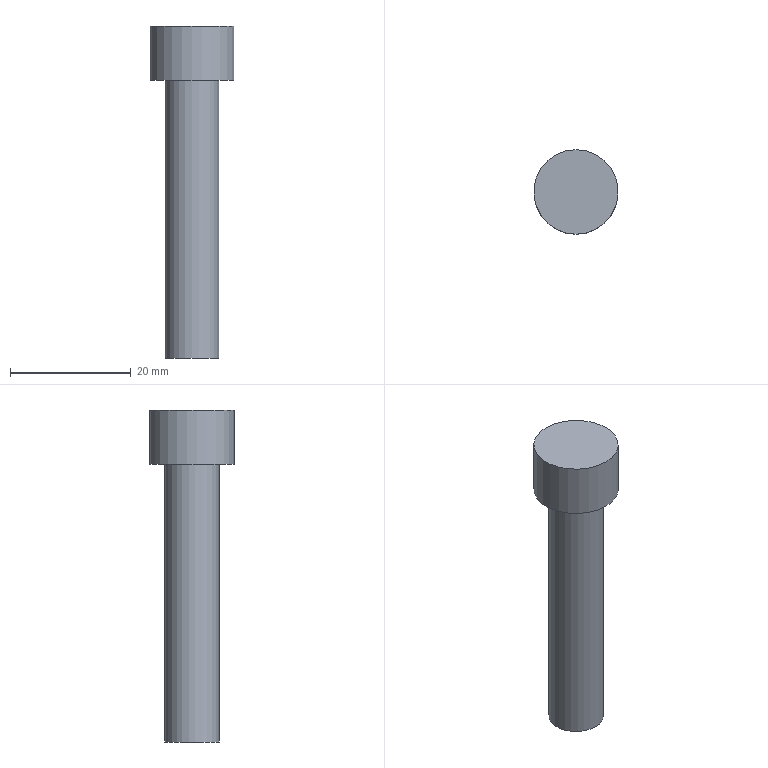Part | STEP file | SOLID | 1 solid | 5 faces | box 14 x 14 x 55 mm | volume 4312 mm3 | plane 3 | cylinder 2 | commonest cylinder face diameters 9 x1 14 x1
STEP:
#1=CARTESIAN_POINT('',(0.,0.,0.));
#2=DIRECTION('',(0.,0.,1.));
#3=DIRECTION('',(1.,0.,0.));
#4=AXIS2_PLACEMENT_3D('',#1,#2,#3);
#5=CARTESIAN_POINT('',(0.,-4.5,-55.));
#6=VERTEX_POINT('',#5);
#7=CARTESIAN_POINT('',(0.,0.,-55.));
#8=DIRECTION('',(0.,0.,1.));
#9=DIRECTION('',(0.,-1.,0.));
#10=AXIS2_PLACEMENT_3D('',#7,#8,#9);
#11=CIRCLE('',#10,4.5);
#12=CARTESIAN_POINT('',(0.,0.,-55.));
#13=DIRECTION('',(0.,0.,1.));
#14=DIRECTION('',(0.,-1.,0.));
#15=AXIS2_PLACEMENT_3D('',#12,#13,#14);
#16=PLANE('',#15);
#17=CARTESIAN_POINT('',(0.,0.));
#18=DIRECTION('',(1.,0.));
#19=AXIS2_PLACEMENT_2D('',#17,#18);
#20=CIRCLE('',#19,4.5);
#21=(GEOMETRIC_REPRESENTATION_CONTEXT(2)PARAMETRIC_REPRESENTATION_CONTEXT()REPRESENTATION_CONTEXT('',''));
#22=DEFINITIONAL_REPRESENTATION('',(#20),#21);
#23=PCURVE('',#16,#22);
#24=CARTESIAN_POINT('',(0.,0.,1.));
#25=DIRECTION('',(0.,0.,1.));
#26=DIRECTION('',(0.,-1.,0.));
#27=AXIS2_PLACEMENT_3D('',#24,#25,#26);
#28=CYLINDRICAL_SURFACE('',#27,4.5);
#29=CARTESIAN_POINT('',(0.,-56.));
#30=DIRECTION('',(1.,0.));
#31=VECTOR('',#30,1.);
#32=LINE('',#29,#31);
#33=(GEOMETRIC_REPRESENTATION_CONTEXT(2)PARAMETRIC_REPRESENTATION_CONTEXT()REPRESENTATION_CONTEXT('',''));
#34=DEFINITIONAL_REPRESENTATION('',(#32),#33);
#35=PCURVE('',#28,#34);
#36=SURFACE_CURVE('',#11,(#23,#35),.PCURVE_S1.);
#37=EDGE_CURVE('',#6,#6,#36,.T.);
#38=ORIENTED_EDGE('',*,*,#37,.F.);
#39=EDGE_LOOP('',(#38));
#40=FACE_BOUND('',#39,.T.);
#41=ADVANCED_FACE('',(#40),#16,.F.);
#42=ORIENTED_EDGE('',*,*,#37,.T.);
#43=CARTESIAN_POINT('',(0.,-4.5,-9.));
#44=VERTEX_POINT('',#43);
#45=CARTESIAN_POINT('',(0.,-4.5,-55.));
#46=CARTESIAN_POINT('',(0.,-4.5,-9.));
#47=B_SPLINE_CURVE_WITH_KNOTS('',1,(#45,#46),.UNSPECIFIED.,.F.,.F.,(2,2),(-56.,-10.),.PIECEWISE_BEZIER_KNOTS.);
#48=CARTESIAN_POINT('',(6.283,0.));
#49=DIRECTION('',(0.,1.));
#50=VECTOR('',#49,1.);
#51=LINE('',#48,#50);
#52=(GEOMETRIC_REPRESENTATION_CONTEXT(2)PARAMETRIC_REPRESENTATION_CONTEXT()REPRESENTATION_CONTEXT('',''));
#53=DEFINITIONAL_REPRESENTATION('',(#51),#52);
#54=PCURVE('',#28,#53);
#55=CARTESIAN_POINT('',(0.,0.));
#56=DIRECTION('',(0.,1.));
#57=VECTOR('',#56,1.);
#58=LINE('',#55,#57);
#59=(GEOMETRIC_REPRESENTATION_CONTEXT(2)PARAMETRIC_REPRESENTATION_CONTEXT()REPRESENTATION_CONTEXT('',''));
#60=DEFINITIONAL_REPRESENTATION('',(#58),#59);
#61=PCURVE('',#28,#60);
#62=SEAM_CURVE('',#47,(#54,#61),.PCURVE_S1.);
#63=EDGE_CURVE('',#6,#44,#62,.T.);
#64=ORIENTED_EDGE('',*,*,#63,.T.);
#65=CARTESIAN_POINT('',(0.,0.,-9.));
#66=DIRECTION('',(0.,0.,1.));
#67=DIRECTION('',(0.,-1.,0.));
#68=AXIS2_PLACEMENT_3D('',#65,#66,#67);
#69=CIRCLE('',#68,4.5);
#70=CARTESIAN_POINT('',(0.,-10.));
#71=DIRECTION('',(1.,0.));
#72=VECTOR('',#71,1.);
#73=LINE('',#70,#72);
#74=(GEOMETRIC_REPRESENTATION_CONTEXT(2)PARAMETRIC_REPRESENTATION_CONTEXT()REPRESENTATION_CONTEXT('',''));
#75=DEFINITIONAL_REPRESENTATION('',(#73),#74);
#76=PCURVE('',#28,#75);
#77=CARTESIAN_POINT('',(0.,0.,-9.));
#78=DIRECTION('',(0.,0.,1.));
#79=DIRECTION('',(0.,-1.,0.));
#80=AXIS2_PLACEMENT_3D('',#77,#78,#79);
#81=PLANE('',#80);
#82=CARTESIAN_POINT('',(0.,0.));
#83=DIRECTION('',(1.,0.));
#84=AXIS2_PLACEMENT_2D('',#82,#83);
#85=CIRCLE('',#84,4.5);
#86=(GEOMETRIC_REPRESENTATION_CONTEXT(2)PARAMETRIC_REPRESENTATION_CONTEXT()REPRESENTATION_CONTEXT('',''));
#87=DEFINITIONAL_REPRESENTATION('',(#85),#86);
#88=PCURVE('',#81,#87);
#89=SURFACE_CURVE('',#69,(#76,#88),.PCURVE_S1.);
#90=EDGE_CURVE('',#44,#44,#89,.T.);
#91=ORIENTED_EDGE('',*,*,#90,.F.);
#92=ORIENTED_EDGE('',*,*,#63,.F.);
#93=EDGE_LOOP('',(#42,#64,#91,#92));
#94=FACE_BOUND('',#93,.T.);
#95=ADVANCED_FACE('',(#94),#28,.T.);
#96=CARTESIAN_POINT('',(0.,-7.,-9.));
#97=VERTEX_POINT('',#96);
#98=CARTESIAN_POINT('',(0.,0.,-9.));
#99=DIRECTION('',(0.,0.,1.));
#100=DIRECTION('',(0.,-1.,0.));
#101=AXIS2_PLACEMENT_3D('',#98,#99,#100);
#102=CIRCLE('',#101,7.);
#103=CARTESIAN_POINT('',(0.,0.));
#104=DIRECTION('',(1.,0.));
#105=AXIS2_PLACEMENT_2D('',#103,#104);
#106=CIRCLE('',#105,7.);
#107=(GEOMETRIC_REPRESENTATION_CONTEXT(2)PARAMETRIC_REPRESENTATION_CONTEXT()REPRESENTATION_CONTEXT('',''));
#108=DEFINITIONAL_REPRESENTATION('',(#106),#107);
#109=PCURVE('',#81,#108);
#110=CARTESIAN_POINT('',(0.,0.,1.));
#111=DIRECTION('',(0.,0.,1.));
#112=DIRECTION('',(0.,-1.,0.));
#113=AXIS2_PLACEMENT_3D('',#110,#111,#112);
#114=CYLINDRICAL_SURFACE('',#113,7.);
#115=CARTESIAN_POINT('',(0.,-10.));
#116=DIRECTION('',(1.,0.));
#117=VECTOR('',#116,1.);
#118=LINE('',#115,#117);
#119=(GEOMETRIC_REPRESENTATION_CONTEXT(2)PARAMETRIC_REPRESENTATION_CONTEXT()REPRESENTATION_CONTEXT('',''));
#120=DEFINITIONAL_REPRESENTATION('',(#118),#119);
#121=PCURVE('',#114,#120);
#122=SURFACE_CURVE('',#102,(#109,#121),.PCURVE_S1.);
#123=EDGE_CURVE('',#97,#97,#122,.T.);
#124=ORIENTED_EDGE('',*,*,#123,.F.);
#125=EDGE_LOOP('',(#124));
#126=FACE_BOUND('',#125,.T.);
#127=ORIENTED_EDGE('',*,*,#90,.T.);
#128=EDGE_LOOP('',(#127));
#129=FACE_BOUND('',#128,.T.);
#130=ADVANCED_FACE('',(#126,#129),#81,.F.);
#131=CARTESIAN_POINT('',(0.,-7.,0.));
#132=VERTEX_POINT('',#131);
#133=CARTESIAN_POINT('',(0.,0.,0.));
#134=DIRECTION('',(0.,0.,1.));
#135=DIRECTION('',(0.,-1.,0.));
#136=AXIS2_PLACEMENT_3D('',#133,#134,#135);
#137=CIRCLE('',#136,7.);
#138=CARTESIAN_POINT('',(0.,0.,0.));
#139=DIRECTION('',(0.,0.,1.));
#140=DIRECTION('',(0.,-1.,0.));
#141=AXIS2_PLACEMENT_3D('',#138,#139,#140);
#142=PLANE('',#141);
#143=CARTESIAN_POINT('',(0.,0.));
#144=DIRECTION('',(1.,0.));
#145=AXIS2_PLACEMENT_2D('',#143,#144);
#146=CIRCLE('',#145,7.);
#147=(GEOMETRIC_REPRESENTATION_CONTEXT(2)PARAMETRIC_REPRESENTATION_CONTEXT()REPRESENTATION_CONTEXT('',''));
#148=DEFINITIONAL_REPRESENTATION('',(#146),#147);
#149=PCURVE('',#142,#148);
#150=CARTESIAN_POINT('',(0.,-1.));
#151=DIRECTION('',(1.,0.));
#152=VECTOR('',#151,1.);
#153=LINE('',#150,#152);
#154=(GEOMETRIC_REPRESENTATION_CONTEXT(2)PARAMETRIC_REPRESENTATION_CONTEXT()REPRESENTATION_CONTEXT('',''));
#155=DEFINITIONAL_REPRESENTATION('',(#153),#154);
#156=PCURVE('',#114,#155);
#157=SURFACE_CURVE('',#137,(#149,#156),.PCURVE_S1.);
#158=EDGE_CURVE('',#132,#132,#157,.T.);
#159=ORIENTED_EDGE('',*,*,#158,.T.);
#160=EDGE_LOOP('',(#159));
#161=FACE_BOUND('',#160,.T.);
#162=ADVANCED_FACE('',(#161),#142,.T.);
#163=ORIENTED_EDGE('',*,*,#158,.F.);
#164=CARTESIAN_POINT('',(0.,-7.,-9.));
#165=CARTESIAN_POINT('',(0.,-7.,0.));
#166=B_SPLINE_CURVE_WITH_KNOTS('',1,(#164,#165),.UNSPECIFIED.,.F.,.F.,(2,2),(-10.,-1.),.PIECEWISE_BEZIER_KNOTS.);
#167=CARTESIAN_POINT('',(0.,0.));
#168=DIRECTION('',(0.,1.));
#169=VECTOR('',#168,1.);
#170=LINE('',#167,#169);
#171=(GEOMETRIC_REPRESENTATION_CONTEXT(2)PARAMETRIC_REPRESENTATION_CONTEXT()REPRESENTATION_CONTEXT('',''));
#172=DEFINITIONAL_REPRESENTATION('',(#170),#171);
#173=PCURVE('',#114,#172);
#174=CARTESIAN_POINT('',(6.283,0.));
#175=DIRECTION('',(0.,1.));
#176=VECTOR('',#175,1.);
#177=LINE('',#174,#176);
#178=(GEOMETRIC_REPRESENTATION_CONTEXT(2)PARAMETRIC_REPRESENTATION_CONTEXT()REPRESENTATION_CONTEXT('',''));
#179=DEFINITIONAL_REPRESENTATION('',(#177),#178);
#180=PCURVE('',#114,#179);
#181=SEAM_CURVE('',#166,(#173,#180),.PCURVE_S1.);
#182=EDGE_CURVE('',#97,#132,#181,.T.);
#183=ORIENTED_EDGE('',*,*,#182,.F.);
#184=ORIENTED_EDGE('',*,*,#123,.T.);
#185=ORIENTED_EDGE('',*,*,#182,.T.);
#186=EDGE_LOOP('',(#163,#183,#184,#185));
#187=FACE_BOUND('',#186,.T.);
#188=ADVANCED_FACE('',(#187),#114,.T.);
#189=CLOSED_SHELL('',(#41,#95,#130,#162,#188));
#190=MANIFOLD_SOLID_BREP('',#189);
#191=(LENGTH_UNIT()NAMED_UNIT(*)SI_UNIT(.MILLI.,.METRE.));
#192=UNCERTAINTY_MEASURE_WITH_UNIT(LENGTH_MEASURE(0.00001),#191,'','');
#193=(NAMED_UNIT(*)PLANE_ANGLE_UNIT()SI_UNIT($,.RADIAN.));
#194=(NAMED_UNIT(*)SI_UNIT($,.STERADIAN.)SOLID_ANGLE_UNIT());
#195=(GEOMETRIC_REPRESENTATION_CONTEXT(3)GLOBAL_UNCERTAINTY_ASSIGNED_CONTEXT((#192))GLOBAL_UNIT_ASSIGNED_CONTEXT((#191,#193,#194))REPRESENTATION_CONTEXT('',''));
#196=ADVANCED_BREP_SHAPE_REPRESENTATION('',(#4,#190),#195);